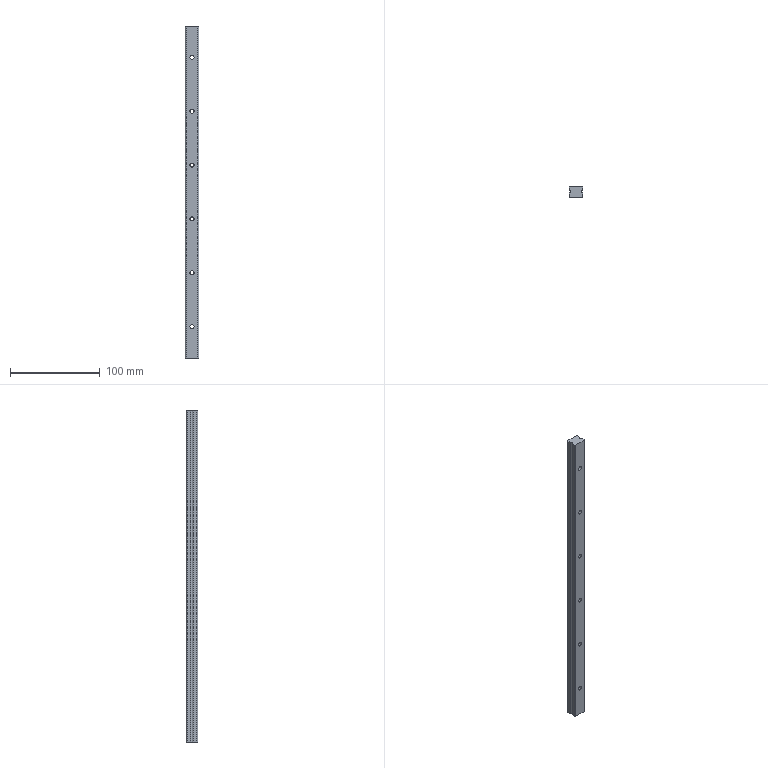Part | STEP file | Rail SSR15XW1SSC1+370LY | 1 solid | 45 faces | box 15 x 12.5 x 370 mm | volume 64350 mm3 | cylinder 31 | plane 14 | commonest cylinder face diameters 4.5 x12 7.5 x12 2 x4 3 x3